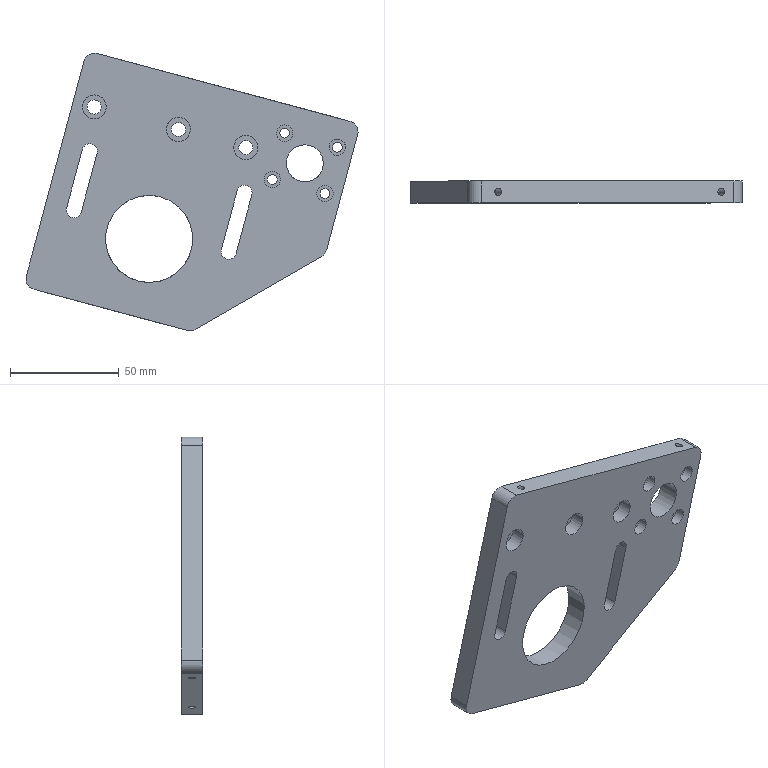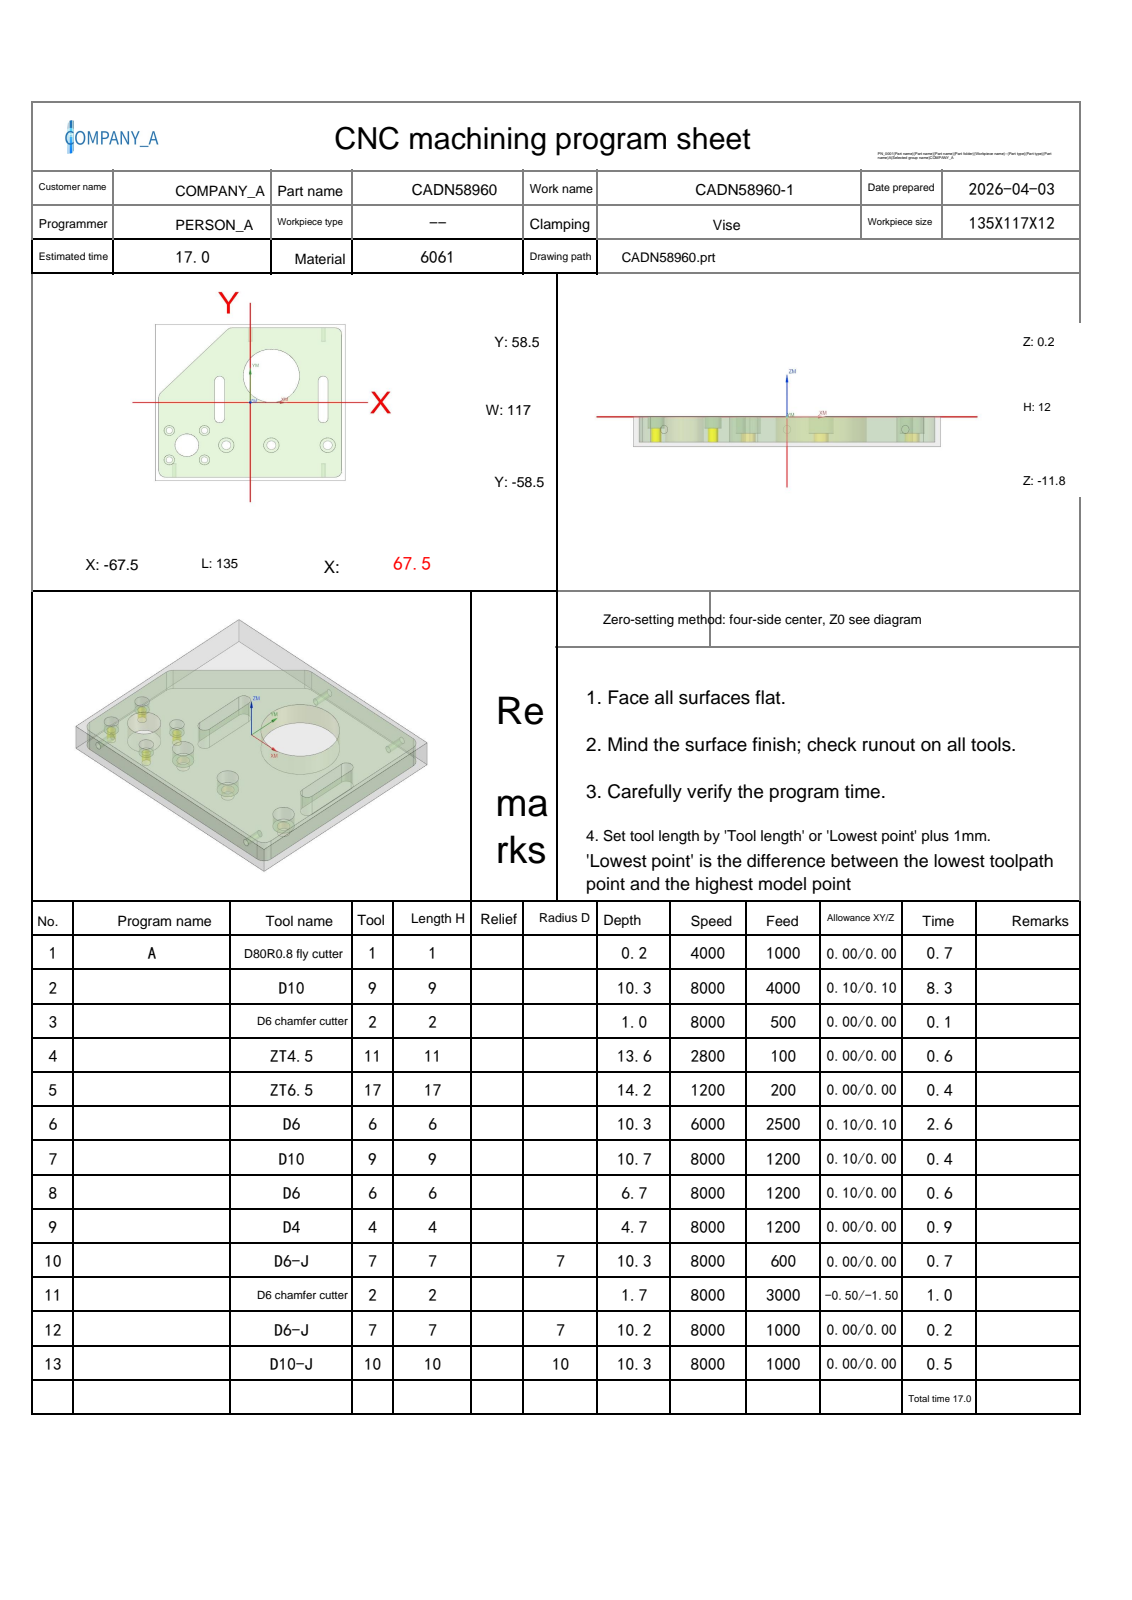NC program | NX | posted by the shop | part box 152.311 x 10 x 127.359 mm
Lines 40 to 980 of 4827:
N2 T09 M06
(D10  D=10. R=0. H=09 ce=0.10 di=0.10)
G00 G90 G54 X8.877 Y31.644 M03 S8000
G43 H09 Z10.2
M08
Z1.5
G02 X8.877 Y31.644 Z1.006 I3.69 J-2.576 F4000.
X8.877 Y31.644 Z.513 I3.69 J-2.576
X8.877 Y31.644 Z.019 I3.69 J-2.576
X8.877 Y31.644 Z-.474 I3.69 J-2.576
X9.115 Y31.955 Z-.481 I3.69 J-2.576
G01 X11.144 Y34.381
G02 X15. Y34.889 I3.856 J-14.392
X29.9 Y19.989 I0.0 J-14.9
X15. Y5.089 I-14.9 J0.0
X.1 Y19.989 I0.0 J14.9
X15. Y34.889 I14.9 J0.0
X16.098 Y34.848 I0.0 J-14.9
X17.014 Y33.997 I-.074 J-.997
G01 X17.925 Y27.835
G03 X18.474 Y27.084 I.989 J.147
G02 X22.9 Y19.989 I-3.474 J-7.095
X15. Y12.089 I-7.9 J0.0
X7.1 Y19.989 I0.0 J7.9
X12.241 Y27.391 I7.9 J0.0
X12.555 Y27.448 I.314 J-.843
X13.398 Y26.862 I0.0 J-.9
G01 X15.831 Y20.335
X15.84 Y20.311
G02 X15.9 Y19.989 I-.84 J-.322
X15. Y19.089 I-.9 J0.0
X14.1 Y19.989 I0.0 J.9
X15. Y20.889 I.9 J0.0
G01 X15.066 Y20.886
G02 X15.53 Y20.716 I-.066 J-.898
G03 X19.65 Y19.375 I4.12 J5.659
X25.309 Y22.255 I0.0 J7.
G01 Z.719
G00 Z3.
G01 X8.877 Y31.644 F6000.
G00 Z1.019
G02 X8.877 Y31.644 Z.526 I3.69 J-2.576 F4000.
X8.877 Y31.644 Z.032 I3.69 J-2.576
X8.877 Y31.644 Z-.462 I3.69 J-2.576
X8.877 Y31.644 Z-.955 I3.69 J-2.576
X9.115 Y31.955 Z-.962 I3.69 J-2.576
G01 X11.144 Y34.381
G02 X15. Y34.889 I3.856 J-14.392
X29.9 Y19.989 I0.0 J-14.9
X15. Y5.089 I-14.9 J0.0
X.1 Y19.989 I0.0 J14.9
X15. Y34.889 I14.9 J0.0
X16.098 Y34.848 I0.0 J-14.9
X17.014 Y33.997 I-.074 J-.997
G01 X17.925 Y27.835
G03 X18.474 Y27.084 I.989 J.147
G02 X22.9 Y19.989 I-3.474 J-7.095
X15. Y12.089 I-7.9 J0.0
X7.1 Y19.989 I0.0 J7.9
X12.241 Y27.391 I7.9 J0.0
X12.555 Y27.448 I.314 J-.843
X13.398 Y26.862 I0.0 J-.9
G01 X15.831 Y20.335
X15.84 Y20.311
G02 X15.9 Y19.989 I-.84 J-.322
X15. Y19.089 I-.9 J0.0
X14.1 Y19.989 I0.0 J.9
X15. Y20.889 I.9 J0.0
G01 X15.066 Y20.886
G02 X15.53 Y20.716 I-.066 J-.898
G03 X19.65 Y19.375 I4.12 J5.659
X25.309 Y22.255 I0.0 J7.
G01 Z.238
G00 Z2.519
G01 X8.877 Y31.644 F6000.
G00 Z.538
G02 X8.877 Y31.644 Z.045 I3.69 J-2.576 F4000.
X8.877 Y31.644 Z-.449 I3.69 J-2.576
X8.877 Y31.644 Z-.942 I3.69 J-2.576
X8.877 Y31.644 Z-1.436 I3.69 J-2.576
X9.115 Y31.955 Z-1.443 I3.69 J-2.576
G01 X11.144 Y34.381
G02 X15. Y34.889 I3.856 J-14.392
X29.9 Y19.989 I0.0 J-14.9
X15. Y5.089 I-14.9 J0.0
X.1 Y19.989 I0.0 J14.9
X15. Y34.889 I14.9 J0.0
X16.098 Y34.848 I0.0 J-14.9
X17.014 Y33.997 I-.074 J-.997
G01 X17.925 Y27.835
G03 X18.474 Y27.084 I.989 J.147
G02 X22.9 Y19.989 I-3.474 J-7.095
X15. Y12.089 I-7.9 J0.0
X7.1 Y19.989 I0.0 J7.9
X12.241 Y27.391 I7.9 J0.0
X12.555 Y27.448 I.314 J-.843
X13.398 Y26.862 I0.0 J-.9
G01 X15.831 Y20.335
X15.84 Y20.311
G02 X15.9 Y19.989 I-.84 J-.322
X15. Y19.089 I-.9 J0.0
X14.1 Y19.989 I0.0 J.9
X15. Y20.889 I.9 J0.0
G01 X15.066 Y20.886
G02 X15.53 Y20.716 I-.066 J-.898
G03 X19.65 Y19.375 I4.12 J5.659
X25.309 Y22.255 I0.0 J7.
G01 Z-.243
G00 Z2.038
G01 X8.877 Y31.644 F6000.
G00 Z.057
G02 X8.877 Y31.644 Z-.436 I3.69 J-2.576 F4000.
X8.877 Y31.644 Z-.93 I3.69 J-2.576
X8.877 Y31.644 Z-1.423 I3.69 J-2.576
X8.877 Y31.644 Z-1.917 I3.69 J-2.576
X9.115 Y31.955 Z-1.924 I3.69 J-2.576
G01 X11.144 Y34.381
G02 X15. Y34.889 I3.856 J-14.392
X29.9 Y19.989 I0.0 J-14.9
X15. Y5.089 I-14.9 J0.0
X.1 Y19.989 I0.0 J14.9
X15. Y34.889 I14.9 J0.0
X16.098 Y34.848 I0.0 J-14.9
X17.014 Y33.997 I-.074 J-.997
G01 X17.925 Y27.835
G03 X18.474 Y27.084 I.989 J.147
G02 X22.9 Y19.989 I-3.474 J-7.095
X15. Y12.089 I-7.9 J0.0
X7.1 Y19.989 I0.0 J7.9
X12.241 Y27.391 I7.9 J0.0
X12.555 Y27.448 I.314 J-.843
X13.398 Y26.862 I0.0 J-.9
G01 X15.831 Y20.335
X15.84 Y20.311
G02 X15.9 Y19.989 I-.84 J-.322
X15. Y19.089 I-.9 J0.0
X14.1 Y19.989 I0.0 J.9
X15. Y20.889 I.9 J0.0
G01 X15.066 Y20.886
G02 X15.53 Y20.716 I-.066 J-.898
G03 X19.65 Y19.375 I4.12 J5.659
X25.309 Y22.255 I0.0 J7.
G01 Z-.724
G00 Z1.557
G01 X8.877 Y31.644 F6000.
G00 Z-.424
G02 X8.877 Y31.644 Z-.917 I3.69 J-2.576 F4000.
X8.877 Y31.644 Z-1.411 I3.69 J-2.576
X8.877 Y31.644 Z-1.904 I3.69 J-2.576
X8.877 Y31.644 Z-2.398 I3.69 J-2.576
X9.115 Y31.955 Z-2.405 I3.69 J-2.576
G01 X11.144 Y34.381
G02 X15. Y34.889 I3.856 J-14.392
X29.9 Y19.989 I0.0 J-14.9
X15. Y5.089 I-14.9 J0.0
X.1 Y19.989 I0.0 J14.9
X15. Y34.889 I14.9 J0.0
X16.098 Y34.848 I0.0 J-14.9
X17.014 Y33.997 I-.074 J-.997
G01 X17.925 Y27.835
G03 X18.474 Y27.084 I.989 J.147
G02 X22.9 Y19.989 I-3.474 J-7.095
X15. Y12.089 I-7.9 J0.0
X7.1 Y19.989 I0.0 J7.9
X12.241 Y27.391 I7.9 J0.0
X12.555 Y27.448 I.314 J-.843
X13.398 Y26.862 I0.0 J-.9
G01 X15.831 Y20.335
X15.84 Y20.311
G02 X15.9 Y19.989 I-.84 J-.322
X15. Y19.089 I-.9 J0.0
X14.1 Y19.989 I0.0 J.9
X15. Y20.889 I.9 J0.0
G01 X15.066 Y20.886
G02 X15.53 Y20.716 I-.066 J-.898
G03 X19.65 Y19.375 I4.12 J5.659
X25.309 Y22.255 I0.0 J7.
G01 Z-1.205
G00 Z1.076
G01 X8.877 Y31.644 F6000.
G00 Z-.905
G02 X8.877 Y31.644 Z-1.398 I3.69 J-2.576 F4000.
X8.877 Y31.644 Z-1.892 I3.69 J-2.576
X8.877 Y31.644 Z-2.385 I3.69 J-2.576
X8.877 Y31.644 Z-2.879 I3.69 J-2.576
X9.115 Y31.955 Z-2.886 I3.69 J-2.576
G01 X11.144 Y34.381
G02 X15. Y34.889 I3.856 J-14.392
X29.9 Y19.989 I0.0 J-14.9
X15. Y5.089 I-14.9 J0.0
X.1 Y19.989 I0.0 J14.9
X15. Y34.889 I14.9 J0.0
X16.098 Y34.848 I0.0 J-14.9
X17.014 Y33.997 I-.074 J-.997
G01 X17.925 Y27.835
G03 X18.474 Y27.084 I.989 J.147
G02 X22.9 Y19.989 I-3.474 J-7.095
X15. Y12.089 I-7.9 J0.0
X7.1 Y19.989 I0.0 J7.9
X12.241 Y27.391 I7.9 J0.0
X12.555 Y27.448 I.314 J-.843
X13.398 Y26.862 I0.0 J-.9
G01 X15.831 Y20.335
X15.84 Y20.311
G02 X15.9 Y19.989 I-.84 J-.322
X15. Y19.089 I-.9 J0.0
X14.1 Y19.989 I0.0 J.9
X15. Y20.889 I.9 J0.0
G01 X15.066 Y20.886
G02 X15.53 Y20.716 I-.066 J-.898
G03 X19.65 Y19.375 I4.12 J5.659
X25.309 Y22.255 I0.0 J7.
G01 Z-1.686
G00 Z.595
G01 X8.877 Y31.644 F6000.
G00 Z-1.386
G02 X8.877 Y31.644 Z-1.879 I3.69 J-2.576 F4000.
X8.877 Y31.644 Z-2.373 I3.69 J-2.576
X8.877 Y31.644 Z-2.866 I3.69 J-2.576
X8.877 Y31.644 Z-3.36 I3.69 J-2.576
X9.115 Y31.955 Z-3.367 I3.69 J-2.576
G01 X11.144 Y34.381
G02 X15. Y34.889 I3.856 J-14.392
X29.9 Y19.989 I0.0 J-14.9
X15. Y5.089 I-14.9 J0.0
X.1 Y19.989 I0.0 J14.9
X15. Y34.889 I14.9 J0.0
X16.098 Y34.848 I0.0 J-14.9
X17.014 Y33.997 I-.074 J-.997
G01 X17.925 Y27.835
G03 X18.474 Y27.084 I.989 J.147
G02 X22.9 Y19.989 I-3.474 J-7.095
X15. Y12.089 I-7.9 J0.0
X7.1 Y19.989 I0.0 J7.9
X12.241 Y27.391 I7.9 J0.0
X12.555 Y27.448 I.314 J-.843
X13.398 Y26.862 I0.0 J-.9
G01 X15.831 Y20.335
X15.84 Y20.311
G02 X15.9 Y19.989 I-.84 J-.322
X15. Y19.089 I-.9 J0.0
X14.1 Y19.989 I0.0 J.9
X15. Y20.889 I.9 J0.0
G01 X15.066 Y20.886
G02 X15.53 Y20.716 I-.066 J-.898
G03 X19.65 Y19.375 I4.12 J5.659
X25.309 Y22.255 I0.0 J7.
G01 Z-2.167
G00 Z.114
G01 X8.877 Y31.644 F6000.
G00 Z-1.867
G02 X8.877 Y31.644 Z-2.36 I3.69 J-2.576 F4000.
X8.877 Y31.644 Z-2.854 I3.69 J-2.576
X8.877 Y31.644 Z-3.347 I3.69 J-2.576
X8.877 Y31.644 Z-3.841 I3.69 J-2.576
X9.115 Y31.955 Z-3.848 I3.69 J-2.576
G01 X11.144 Y34.381
G02 X15. Y34.889 I3.856 J-14.392
X29.9 Y19.989 I0.0 J-14.9
X15. Y5.089 I-14.9 J0.0
X.1 Y19.989 I0.0 J14.9
X15. Y34.889 I14.9 J0.0
X16.098 Y34.848 I0.0 J-14.9
X17.014 Y33.997 I-.074 J-.997
G01 X17.925 Y27.835
G03 X18.474 Y27.084 I.989 J.147
G02 X22.9 Y19.989 I-3.474 J-7.095
X15. Y12.089 I-7.9 J0.0
X7.1 Y19.989 I0.0 J7.9
X12.241 Y27.391 I7.9 J0.0
X12.555 Y27.448 I.314 J-.843
X13.398 Y26.862 I0.0 J-.9
G01 X15.831 Y20.335
X15.84 Y20.311
G02 X15.9 Y19.989 I-.84 J-.322
X15. Y19.089 I-.9 J0.0
X14.1 Y19.989 I0.0 J.9
X15. Y20.889 I.9 J0.0
G01 X15.066 Y20.886
G02 X15.53 Y20.716 I-.066 J-.898
G03 X19.65 Y19.375 I4.12 J5.659
X25.309 Y22.255 I0.0 J7.
G01 Z-2.648
G00 Z-.367
G01 X8.877 Y31.644 F6000.
G00 Z-2.348
G02 X8.877 Y31.644 Z-2.841 I3.69 J-2.576 F4000.
X8.877 Y31.644 Z-3.335 I3.69 J-2.576
X8.877 Y31.644 Z-3.828 I3.69 J-2.576
X8.877 Y31.644 Z-4.322 I3.69 J-2.576
X9.115 Y31.955 Z-4.329 I3.69 J-2.576
G01 X11.144 Y34.381
G02 X15. Y34.889 I3.856 J-14.392
X29.9 Y19.989 I0.0 J-14.9
X15. Y5.089 I-14.9 J0.0
X.1 Y19.989 I0.0 J14.9
X15. Y34.889 I14.9 J0.0
X16.098 Y34.848 I0.0 J-14.9
X17.014 Y33.997 I-.074 J-.997
G01 X17.925 Y27.835
G03 X18.474 Y27.084 I.989 J.147
G02 X22.9 Y19.989 I-3.474 J-7.095
X15. Y12.089 I-7.9 J0.0
X7.1 Y19.989 I0.0 J7.9
X12.241 Y27.391 I7.9 J0.0
X12.555 Y27.448 I.314 J-.843
X13.398 Y26.862 I0.0 J-.9
G01 X15.831 Y20.335
X15.84 Y20.311
G02 X15.9 Y19.989 I-.84 J-.322
X15. Y19.089 I-.9 J0.0
X14.1 Y19.989 I0.0 J.9
X15. Y20.889 I.9 J0.0
G01 X15.066 Y20.886
G02 X15.53 Y20.716 I-.066 J-.898
G03 X19.65 Y19.375 I4.12 J5.659
X25.309 Y22.255 I0.0 J7.
G01 Z-3.129
G00 Z-.848
G01 X8.877 Y31.644 F6000.
G00 Z-2.829
G02 X8.877 Y31.644 Z-3.322 I3.69 J-2.576 F4000.
X8.877 Y31.644 Z-3.816 I3.69 J-2.576
X8.877 Y31.644 Z-4.309 I3.69 J-2.576
X8.877 Y31.644 Z-4.803 I3.69 J-2.576
X9.115 Y31.955 Z-4.81 I3.69 J-2.576
G01 X11.144 Y34.381
G02 X15. Y34.889 I3.856 J-14.392
X29.9 Y19.989 I0.0 J-14.9
X15. Y5.089 I-14.9 J0.0
X.1 Y19.989 I0.0 J14.9
X15. Y34.889 I14.9 J0.0
X16.098 Y34.848 I0.0 J-14.9
X17.014 Y33.997 I-.074 J-.997
G01 X17.925 Y27.835
G03 X18.474 Y27.084 I.989 J.147
G02 X22.9 Y19.989 I-3.474 J-7.095
X15. Y12.089 I-7.9 J0.0
X7.1 Y19.989 I0.0 J7.9
X12.241 Y27.391 I7.9 J0.0
X12.555 Y27.448 I.314 J-.843
X13.398 Y26.862 I0.0 J-.9
G01 X15.831 Y20.335
X15.84 Y20.311
G02 X15.9 Y19.989 I-.84 J-.322
X15. Y19.089 I-.9 J0.0
X14.1 Y19.989 I0.0 J.9
X15. Y20.889 I.9 J0.0
G01 X15.066 Y20.886
G02 X15.53 Y20.716 I-.066 J-.898
G03 X19.65 Y19.375 I4.12 J5.659
X25.309 Y22.255 I0.0 J7.
G01 Z-3.61
G00 Z-1.329
G01 X8.877 Y31.644 F6000.
G00 Z-3.31
G02 X8.877 Y31.644 Z-3.803 I3.69 J-2.576 F4000.
X8.877 Y31.644 Z-4.297 I3.69 J-2.576
X8.877 Y31.644 Z-4.79 I3.69 J-2.576
X8.877 Y31.644 Z-5.284 I3.69 J-2.576
X9.115 Y31.955 Z-5.29 I3.69 J-2.576
G01 X11.144 Y34.381
G02 X15. Y34.889 I3.856 J-14.392
X29.9 Y19.989 I0.0 J-14.9
X15. Y5.089 I-14.9 J0.0
X.1 Y19.989 I0.0 J14.9
X15. Y34.889 I14.9 J0.0
X16.098 Y34.848 I0.0 J-14.9
X17.014 Y33.997 I-.074 J-.997
G01 X17.925 Y27.835
G03 X18.474 Y27.084 I.989 J.147
G02 X22.9 Y19.989 I-3.474 J-7.095
X15. Y12.089 I-7.9 J0.0
X7.1 Y19.989 I0.0 J7.9
X12.241 Y27.391 I7.9 J0.0
X12.555 Y27.448 I.314 J-.843
X13.398 Y26.862 I0.0 J-.9
G01 X15.831 Y20.335
X15.84 Y20.311
G02 X15.9 Y19.989 I-.84 J-.322
X15. Y19.089 I-.9 J0.0
X14.1 Y19.989 I0.0 J.9
X15. Y20.889 I.9 J0.0
G01 X15.066 Y20.886
G02 X15.53 Y20.716 I-.066 J-.898
G03 X19.65 Y19.375 I4.12 J5.659
X25.309 Y22.255 I0.0 J7.
G01 Z-4.09
G00 Z-1.81
G01 X8.877 Y31.644 F6000.
G00 Z-3.79
G02 X8.877 Y31.644 Z-4.284 I3.69 J-2.576 F4000.
X8.877 Y31.644 Z-4.778 I3.69 J-2.576
X8.877 Y31.644 Z-5.271 I3.69 J-2.576
X8.877 Y31.644 Z-5.765 I3.69 J-2.576
X9.115 Y31.955 Z-5.771 I3.69 J-2.576
G01 X11.144 Y34.381
G02 X15. Y34.889 I3.856 J-14.392
X29.9 Y19.989 I0.0 J-14.9
X15. Y5.089 I-14.9 J0.0
X.1 Y19.989 I0.0 J14.9
X15. Y34.889 I14.9 J0.0
X16.098 Y34.848 I0.0 J-14.9
X17.014 Y33.997 I-.074 J-.997
G01 X17.925 Y27.835
G03 X18.474 Y27.084 I.989 J.147
G02 X22.9 Y19.989 I-3.474 J-7.095
X15. Y12.089 I-7.9 J0.0
X7.1 Y19.989 I0.0 J7.9
X12.241 Y27.391 I7.9 J0.0
X12.555 Y27.448 I.314 J-.843
X13.398 Y26.862 I0.0 J-.9
G01 X15.831 Y20.335
X15.84 Y20.311
G02 X15.9 Y19.989 I-.84 J-.322
X15. Y19.089 I-.9 J0.0
X14.1 Y19.989 I0.0 J.9
X15. Y20.889 I.9 J0.0
G01 X15.066 Y20.886
G02 X15.53 Y20.716 I-.066 J-.898
G03 X19.65 Y19.375 I4.12 J5.659
X25.309 Y22.255 I0.0 J7.
G01 Z-4.571
G00 Z-2.29
G01 X8.877 Y31.644 F6000.
G00 Z-4.271
G02 X8.877 Y31.644 Z-4.765 I3.69 J-2.576 F4000.
X8.877 Y31.644 Z-5.258 I3.69 J-2.576
X8.877 Y31.644 Z-5.752 I3.69 J-2.576
X8.877 Y31.644 Z-6.246 I3.69 J-2.576
X9.115 Y31.955 Z-6.252 I3.69 J-2.576
G01 X11.144 Y34.381
G02 X15. Y34.889 I3.856 J-14.392
X29.9 Y19.989 I0.0 J-14.9
X15. Y5.089 I-14.9 J0.0
X.1 Y19.989 I0.0 J14.9
X15. Y34.889 I14.9 J0.0
X16.098 Y34.848 I0.0 J-14.9
X17.014 Y33.997 I-.074 J-.997
G01 X17.925 Y27.835
G03 X18.474 Y27.084 I.989 J.147
G02 X22.9 Y19.989 I-3.474 J-7.095
X15. Y12.089 I-7.9 J0.0
X7.1 Y19.989 I0.0 J7.9
X12.241 Y27.391 I7.9 J0.0
X12.555 Y27.448 I.314 J-.843
X13.398 Y26.862 I0.0 J-.9
G01 X15.831 Y20.335
X15.84 Y20.311
G02 X15.9 Y19.989 I-.84 J-.322
X15. Y19.089 I-.9 J0.0
X14.1 Y19.989 I0.0 J.9
X15. Y20.889 I.9 J0.0
G01 X15.066 Y20.886
G02 X15.53 Y20.716 I-.066 J-.898
G03 X19.65 Y19.375 I4.12 J5.659
X25.309 Y22.255 I0.0 J7.
G01 Z-5.052
G00 Z-2.771
G01 X8.877 Y31.644 F6000.
G00 Z-4.752
G02 X8.877 Y31.644 Z-5.246 I3.69 J-2.576 F4000.
X8.877 Y31.644 Z-5.739 I3.69 J-2.576
X8.877 Y31.644 Z-6.233 I3.69 J-2.576
X8.877 Y31.644 Z-6.727 I3.69 J-2.576
X9.115 Y31.955 Z-6.733 I3.69 J-2.576
G01 X11.144 Y34.381
G02 X15. Y34.889 I3.856 J-14.392
X29.9 Y19.989 I0.0 J-14.9
X15. Y5.089 I-14.9 J0.0
X.1 Y19.989 I0.0 J14.9
X15. Y34.889 I14.9 J0.0
X16.098 Y34.848 I0.0 J-14.9
X17.014 Y33.997 I-.074 J-.997
G01 X17.925 Y27.835
G03 X18.474 Y27.084 I.989 J.147
G02 X22.9 Y19.989 I-3.474 J-7.095
X15. Y12.089 I-7.9 J0.0
X7.1 Y19.989 I0.0 J7.9
X12.241 Y27.391 I7.9 J0.0
X12.555 Y27.448 I.314 J-.843
X13.398 Y26.862 I0.0 J-.9
G01 X15.831 Y20.335
X15.84 Y20.311
G02 X15.9 Y19.989 I-.84 J-.322
X15. Y19.089 I-.9 J0.0
X14.1 Y19.989 I0.0 J.9
X15. Y20.889 I.9 J0.0
G01 X15.066 Y20.886
G02 X15.53 Y20.716 I-.066 J-.898
G03 X19.65 Y19.375 I4.12 J5.659
X25.309 Y22.255 I0.0 J7.
G01 Z-5.533
G00 Z-3.252
G01 X8.877 Y31.644 F6000.
G00 Z-5.233
G02 X8.877 Y31.644 Z-5.727 I3.69 J-2.576 F4000.
X8.877 Y31.644 Z-6.22 I3.69 J-2.576
X8.877 Y31.644 Z-6.714 I3.69 J-2.576
X8.877 Y31.644 Z-7.207 I3.69 J-2.576
X9.115 Y31.955 Z-7.214 I3.69 J-2.576
G01 X11.144 Y34.381
G02 X15. Y34.889 I3.856 J-14.392
X29.9 Y19.989 I0.0 J-14.9
X15. Y5.089 I-14.9 J0.0
X.1 Y19.989 I0.0 J14.9
X15. Y34.889 I14.9 J0.0
X16.098 Y34.848 I0.0 J-14.9
X17.014 Y33.997 I-.074 J-.997
G01 X17.925 Y27.835
G03 X18.474 Y27.084 I.989 J.147
G02 X22.9 Y19.989 I-3.474 J-7.095
X15. Y12.089 I-7.9 J0.0
X7.1 Y19.989 I0.0 J7.9
X12.241 Y27.391 I7.9 J0.0
X12.555 Y27.448 I.314 J-.843
X13.398 Y26.862 I0.0 J-.9
G01 X15.831 Y20.335
X15.84 Y20.311
G02 X15.9 Y19.989 I-.84 J-.322
X15. Y19.089 I-.9 J0.0
X14.1 Y19.989 I0.0 J.9
X15. Y20.889 I.9 J0.0
G01 X15.066 Y20.886
G02 X15.53 Y20.716 I-.066 J-.898
G03 X19.65 Y19.375 I4.12 J5.659
X25.309 Y22.255 I0.0 J7.
G01 Z-6.014
G00 Z-3.733
G01 X8.877 Y31.644 F6000.
G00 Z-5.714
G02 X8.877 Y31.644 Z-6.208 I3.69 J-2.576 F4000.
X8.877 Y31.644 Z-6.701 I3.69 J-2.576
X8.877 Y31.644 Z-7.195 I3.69 J-2.576
X8.877 Y31.644 Z-7.688 I3.69 J-2.576
X9.115 Y31.955 Z-7.695 I3.69 J-2.576
G01 X11.144 Y34.381
G02 X15. Y34.889 I3.856 J-14.392
X29.9 Y19.989 I0.0 J-14.9
X15. Y5.089 I-14.9 J0.0
X.1 Y19.989 I0.0 J14.9
X15. Y34.889 I14.9 J0.0
X16.098 Y34.848 I0.0 J-14.9
X17.014 Y33.997 I-.074 J-.997
G01 X17.925 Y27.835
G03 X18.474 Y27.084 I.989 J.147
G02 X22.9 Y19.989 I-3.474 J-7.095
X15. Y12.089 I-7.9 J0.0
X7.1 Y19.989 I0.0 J7.9
X12.241 Y27.391 I7.9 J0.0
X12.555 Y27.448 I.314 J-.843
X13.398 Y26.862 I0.0 J-.9
G01 X15.831 Y20.335
X15.84 Y20.311
G02 X15.9 Y19.989 I-.84 J-.322
X15. Y19.089 I-.9 J0.0
X14.1 Y19.989 I0.0 J.9
X15. Y20.889 I.9 J0.0
G01 X15.066 Y20.886
G02 X15.53 Y20.716 I-.066 J-.898
G03 X19.65 Y19.375 I4.12 J5.659
X25.309 Y22.255 I0.0 J7.
G01 Z-6.495
G00 Z-4.214
G01 X8.877 Y31.644 F6000.
G00 Z-6.195
G02 X8.877 Y31.644 Z-6.689 I3.69 J-2.576 F4000.
X8.877 Y31.644 Z-7.182 I3.69 J-2.576
X8.877 Y31.644 Z-7.676 I3.69 J-2.576
X8.877 Y31.644 Z-8.169 I3.69 J-2.576
X9.115 Y31.955 Z-8.176 I3.69 J-2.576
G01 X11.144 Y34.381
G02 X15. Y34.889 I3.856 J-14.392
X29.9 Y19.989 I0.0 J-14.9
X15. Y5.089 I-14.9 J0.0
X.1 Y19.989 I0.0 J14.9
X15. Y34.889 I14.9 J0.0
X16.098 Y34.848 I0.0 J-14.9
X17.014 Y33.997 I-.074 J-.997
G01 X17.925 Y27.835
G03 X18.474 Y27.084 I.989 J.147
G02 X22.9 Y19.989 I-3.474 J-7.095
X15. Y12.089 I-7.9 J0.0
X7.1 Y19.989 I0.0 J7.9
X12.241 Y27.391 I7.9 J0.0
X12.555 Y27.448 I.314 J-.843
X13.398 Y26.862 I0.0 J-.9
G01 X15.831 Y20.335
X15.84 Y20.311
G02 X15.9 Y19.989 I-.84 J-.322
X15. Y19.089 I-.9 J0.0
X14.1 Y19.989 I0.0 J.9
X15. Y20.889 I.9 J0.0
G01 X15.066 Y20.886
G02 X15.53 Y20.716 I-.066 J-.898
G03 X19.65 Y19.375 I4.12 J5.659
X25.309 Y22.255 I0.0 J7.
G01 Z-6.976
G00 Z-4.695
G01 X8.877 Y31.644 F6000.
G00 Z-6.676
G02 X8.877 Y31.644 Z-7.17 I3.69 J-2.576 F4000.
X8.877 Y31.644 Z-7.663 I3.69 J-2.576
X8.877 Y31.644 Z-8.157 I3.69 J-2.576
X8.877 Y31.644 Z-8.65 I3.69 J-2.576
X9.115 Y31.955 Z-8.657 I3.69 J-2.576
G01 X11.144 Y34.381
G02 X15. Y34.889 I3.856 J-14.392
X29.9 Y19.989 I0.0 J-14.9
X15. Y5.089 I-14.9 J0.0
X.1 Y19.989 I0.0 J14.9
X15. Y34.889 I14.9 J0.0
X16.098 Y34.848 I0.0 J-14.9
X17.014 Y33.997 I-.074 J-.997
G01 X17.925 Y27.835
G03 X18.474 Y27.084 I.989 J.147
G02 X22.9 Y19.989 I-3.474 J-7.095
X15. Y12.089 I-7.9 J0.0
X7.1 Y19.989 I0.0 J7.9
X12.241 Y27.391 I7.9 J0.0
X12.555 Y27.448 I.314 J-.843
X13.398 Y26.862 I0.0 J-.9
G01 X15.831 Y20.335
X15.84 Y20.311
G02 X15.9 Y19.989 I-.84 J-.322
X15. Y19.089 I-.9 J0.0
X14.1 Y19.989 I0.0 J.9
X15. Y20.889 I.9 J0.0
G01 X15.066 Y20.886
G02 X15.53 Y20.716 I-.066 J-.898
G03 X19.65 Y19.375 I4.12 J5.659
X25.309 Y22.255 I0.0 J7.
G01 Z-7.457
G00 Z-5.176
G01 X8.877 Y31.644 F6000.
G00 Z-7.157
G02 X8.877 Y31.644 Z-7.651 I3.69 J-2.576 F4000.
X8.877 Y31.644 Z-8.144 I3.69 J-2.576
X8.877 Y31.644 Z-8.638 I3.69 J-2.576
X8.877 Y31.644 Z-9.131 I3.69 J-2.576
X9.115 Y31.955 Z-9.138 I3.69 J-2.576
G01 X11.144 Y34.381
G02 X15. Y34.889 I3.856 J-14.392
X29.9 Y19.989 I0.0 J-14.9
X15. Y5.089 I-14.9 J0.0
X.1 Y19.989 I0.0 J14.9
X15. Y34.889 I14.9 J0.0
X16.098 Y34.848 I0.0 J-14.9
X17.014 Y33.997 I-.074 J-.997
G01 X17.925 Y27.835
G03 X18.474 Y27.084 I.989 J.147
G02 X22.9 Y19.989 I-3.474 J-7.095
X15. Y12.089 I-7.9 J0.0
X7.1 Y19.989 I0.0 J7.9
X12.241 Y27.391 I7.9 J0.0
X12.555 Y27.448 I.314 J-.843
X13.398 Y26.862 I0.0 J-.9
G01 X15.831 Y20.335
X15.84 Y20.311
G02 X15.9 Y19.989 I-.84 J-.322
X15. Y19.089 I-.9 J0.0
X14.1 Y19.989 I0.0 J.9
X15. Y20.889 I.9 J0.0
G01 X15.066 Y20.886
G02 X15.53 Y20.716 I-.066 J-.898
G03 X19.65 Y19.375 I4.12 J5.659
X25.309 Y22.255 I0.0 J7.
G01 Z-7.938
G00 Z-5.657
G01 X8.877 Y31.644 F6000.
G00 Z-7.638
G02 X8.877 Y31.644 Z-8.132 I3.69 J-2.576 F4000.
X8.877 Y31.644 Z-8.625 I3.69 J-2.576
X8.877 Y31.644 Z-9.119 I3.69 J-2.576
X8.877 Y31.644 Z-9.612 I3.69 J-2.576
X9.115 Y31.955 Z-9.619 I3.69 J-2.576
G01 X11.144 Y34.381
G02 X15. Y34.889 I3.856 J-14.392
X29.9 Y19.989 I0.0 J-14.9
X15. Y5.089 I-14.9 J0.0
X.1 Y19.989 I0.0 J14.9
X15. Y34.889 I14.9 J0.0
X16.098 Y34.848 I0.0 J-14.9
X17.014 Y33.997 I-.074 J-.997
G01 X17.925 Y27.835
G03 X18.474 Y27.084 I.989 J.147
G02 X22.9 Y19.989 I-3.474 J-7.095
X15. Y12.089 I-7.9 J0.0
X7.1 Y19.989 I0.0 J7.9
X12.241 Y27.391 I7.9 J0.0
X12.555 Y27.448 I.314 J-.843
X13.398 Y26.862 I0.0 J-.9
G01 X15.831 Y20.335
X15.84 Y20.311
G02 X15.9 Y19.989 I-.84 J-.322
X15. Y19.089 I-.9 J0.0
X14.1 Y19.989 I0.0 J.9
X15. Y20.889 I.9 J0.0
G01 X15.066 Y20.886
G02 X15.53 Y20.716 I-.066 J-.898
G03 X19.65 Y19.375 I4.12 J5.659
X25.309 Y22.255 I0.0 J7.
G01 Z-8.419
G00 Z-6.138
G01 X8.877 Y31.644 F6000.
G00 Z-8.119
G02 X8.877 Y31.644 Z-8.613 I3.69 J-2.576 F4000.
X8.877 Y31.644 Z-9.106 I3.69 J-2.576
X8.877 Y31.644 Z-9.6 I3.69 J-2.576
X8.877 Y31.644 Z-10.093 I3.69 J-2.576
X9.115 Y31.955 Z-10.1 I3.69 J-2.576
G01 X11.144 Y34.381
G02 X15. Y34.889 I3.856 J-14.392
X29.9 Y19.989 I0.0 J-14.9
X15. Y5.089 I-14.9 J0.0
X.1 Y19.989 I0.0 J14.9
X15. Y34.889 I14.9 J0.0
X16.098 Y34.848 I0.0 J-14.9
X17.014 Y33.997 I-.074 J-.997
G01 X17.925 Y27.835
G03 X18.474 Y27.084 I.989 J.147
G02 X22.9 Y19.989 I-3.474 J-7.095
X15. Y12.089 I-7.9 J0.0
X7.1 Y19.989 I0.0 J7.9
X12.171 Y27.365 I7.9 J0.0
X12.493 Y27.424 I.322 J-.84
X13.357 Y26.775 I0.0 J-.9
G01 X14.72 Y22.081
G03 X15.607 Y20.653 I2.987 J.867
G02 X15.9 Y19.989 I-.607 J-.664
X15. Y19.089 I-.9 J0.0
X14.1 Y19.989 I0.0 J.9
X15. Y20.889 I.9 J0.0
G01 X15.066 Y20.886
G02 X15.53 Y20.716 I-.066 J-.898
G03 X19.65 Y19.375 I4.12 J5.659
X25.309 Y22.255 I0.0 J7.
G01 Z-8.9
G00 Z10.2
X-57.175 Y70.5
Z.719
G01 Z-.481
Y66.
G03 X-50.175 Y59. I7. J0.0
G01 X-21.036
X-20.904 Y59.132
G02 X-12.772 Y62.5 I8.132 J-8.132
G01 X60.
G02 X71.5 Y51. I0.0 J-11.5
G01 Y23.495
Y4.133
Y-48.811
Y-51.
G02 X60.84 Y-62.469 I-11.5 J0.0
X59.999 Y-62.5 I-.841 J11.47
G01 X59.952
X-60.
G02 X-71.5 Y-51. I0.0 J11.5
G01 Y-39.916
Y3.772
G02 X-68.132 Y11.904 I11.5 J0.0
G01 X-68. Y12.036
Y58.5
G02 X-67.5 Y59. I.5 J0.0
G01 X-45.175
G02 X-44.203 Y58.238 I0.0 J-1.
G01 X-42.861 Y52.762
G03 X-41.89 Y52. I.971 J.238
G01 X-30.447
G02 X-29.45 Y51. I-.003 J-1.
X-29.74 Y50.295 I-1. J0.0
G01 X-34.715 Y45.32
G02 X-35.422 Y45.027 I-.707 J.707
G01 X-35.528 Y45.033
X-37.498 Y45.243
X-37.604 Y45.248
G03 X-37.986 Y45.172 I0.0 J-1.
G01 X-43.067 Y43.068
G02 X-44.023 Y42.878 I-.957 J2.31
X-46.523 Y45.378 I0.0 J2.5
X-44.98 Y47.687 I2.5 J0.0
G01 X-38.846 Y50.228
G02 X-37.889 Y50.418 I.957 J-2.31
X-35.389 Y47.918 I0.0 J-2.5
X-35.975 Y46.31 I-2.5 J0.0
G03 X-36.209 Y45.716 I.766 J-.643
G01 X-36.287 Y44.115
G02 X-36.579 Y43.457 I-.999 J.049
G01 X-58.947 Y21.089
G03 X-59.175 Y20.538 I.551 J-.551
X-59.13 Y20.277 I.779 J0.0
G01 X-58.998 Y19.906
G03 X-58.602 Y19.627 I.396 J.141
X-58.305 Y19.75 I0.0 J.42
G01 X-47.115 Y30.941
X-45.355 Y32.701
X-19.914 Y58.142
G02 X-12.772 Y61.1 I7.142 J-7.142
G01 X60.
G02 X70.1 Y51. I0.0 J-10.1
G01 Y23.495
Y4.133
Y-48.811
Y-51.
G02 X60.738 Y-61.073 I-10.1 J0.0
X59.999 Y-61.1 I-.739 J10.074
G01 X59.955
X-60.
G02 X-70.1 Y-51. I0.0 J10.1
G01 Y-39.916
Y3.772
G02 X-67.142 Y10.914 I10.1 J0.0
G01 X-58.305 Y19.75
G03 X-58.182 Y20.047 I-.297 J.297
X-58.461 Y20.443 I-.42 J0.0
G01 X-59.084 Y20.665
X-59.218 Y20.688
G03 X-59.441 Y20.62 I0.0 J-.4
G02 X-60. Y20.45 I-.559 J.829
X-61. Y21.447 I0.0 J1.
G01 Y28.482
G02 X-60.628 Y29.26 I1. J0.0
G01 X-59.087 Y30.505
G03 X-58.792 Y30.9 I-.628 J.778
G01 X-56.687 Y35.98
G02 X-54.378 Y37.523 I2.31 J-.957
X-51.878 Y35.023 I0.0 J-2.5
X-52.068 Y34.067 I-2.5 J0.0
G01 X-54.609 Y27.933
G02 X-56.918 Y26.389 I-2.31 J.957
X-59.409 Y28.673 I0.0 J2.5
G03 X-59.664 Y29.258 I-.996 J-.086
G01 X-60.741 Y30.446
G02 X-61. Y31.118 I.741 J.672
G01 Y51.003
G02 X-60.003 Y52. I1. J-.003
G01 X-48.594
G02 X-47.598 Y51.084 I0.0 J-1.
G01 X-47.132 Y45.506
G03 X-46.743 Y44.795 I.997 J.084
G02 X-46.349 Y44. I-.607 J-.795
X-46.64 Y43.295 I-1. J0.0
G01 X-52.295 Y37.64
G02 X-53. Y37.349 I-.705 J.71
X-54. Y38.346 I0.0 J1.
G01 Y44.003
G02 X-53.003 Y45. I1. J-.003
G01 X-47.346
G02 X-47.087 Y44.965 I-.003 J-1.
X-46.656 Y44.721 I-.262 J-.965
G03 X-41.807 Y42.769 I4.85 J5.048
X-36.759 Y44.919 I0.0 J7.
G01 Y70.5
Z.719
G00 Z3.
G01 X-57.175 F6000.
G00 Z.238
G01 Z-.962 F4000.
Y66.
G03 X-50.175 Y59. I7. J0.0
G01 X-21.036
X-20.904 Y59.132
G02 X-12.772 Y62.5 I8.132 J-8.132
G01 X60.
G02 X71.5 Y51. I0.0 J-11.5
G01 Y-51.
G02 X60.839 Y-62.469 I-11.5 J0.0
X59.999 Y-62.5 I-.841 J11.471
G01 X59.952
X-60.
G02 X-71.5 Y-51. I0.0 J11.5
G01 Y3.772
G02 X-68.132 Y11.904 I11.5 J0.0
G01 X-68. Y12.036
Y58.5
G02 X-67.5 Y59. I.5 J0.0
G01 X-45.175
G02 X-44.203 Y58.238 I0.0 J-1.
G01 X-42.861 Y52.762
G03 X-41.89 Y52. I.971 J.238
G01 X-30.446
G02 X-29.45 Y51. I-.003 J-1.
X-29.74 Y50.295 I-1. J0.0
G01 X-34.715 Y45.32
G02 X-35.422 Y45.027 I-.707 J.707
G01 X-35.528 Y45.033
X-37.498 Y45.243
X-37.604 Y45.248
G03 X-37.986 Y45.172 I0.0 J-1.
G01 X-43.067 Y43.068
G02 X-44.023 Y42.878 I-.957 J2.31
X-46.523 Y45.378 I0.0 J2.5
X-44.98 Y47.687 I2.5 J0.0
G01 X-38.846 Y50.228
G02 X-37.889 Y50.418 I.957 J-2.31
X-35.389 Y47.918 I0.0 J-2.5
X-35.975 Y46.31 I-2.5 J0.0
G03 X-36.209 Y45.716 I.766 J-.643
G01 X-36.287 Y44.115
G02 X-36.579 Y43.457 I-.999 J.049
G01 X-52.457 Y27.579
G02 X-53.115 Y27.287 I-.707 J.707
G01 X-54.716 Y27.209
G03 X-55.31 Y26.976 I.049 J-.999
G02 X-56.918 Y26.389 I-1.609 J1.914
X-59.418 Y28.889 I0.0 J2.5
X-59.228 Y29.846 I2.5 J0.0
G01 X-56.687 Y35.98
G02 X-54.378 Y37.523 I2.31 J-.957
X-51.878 Y35.023 I0.0 J-2.5
X-52.068 Y34.067 I-2.5 J0.0
G01 X-54.172 Y28.986
G03 X-54.248 Y28.604 I.924 J-.383
G01 X-54.243 Y28.498
X-54.033 Y26.528
X-54.027 Y26.422
G02 X-54.32 Y25.715 I-1. J0.0
G01 X-58.947 Y21.088
G03 X-59.175 Y20.538 I.551 J-.551
X-59.13 Y20.276 I.779 J0.0
G01 X-58.998 Y19.906
G03 X-58.602 Y19.627 I.396 J.141
X-58.305 Y19.75 I0.0 J.42
G01 X-19.914 Y58.142
G02 X-12.772 Y61.1 I7.142 J-7.142
G01 X60.
G02 X70.1 Y51. I0.0 J-10.1
G01 Y-51.
G02 X60.737 Y-61.073 I-10.1 J0.0
X59.999 Y-61.1 I-.738 J10.074
G01 X59.955
X-60.
G02 X-70.1 Y-51. I0.0 J10.1
G01 Y3.772
G02 X-67.142 Y10.914 I10.1 J0.0
G01 X-58.305 Y19.75
G03 X-58.182 Y20.047 I-.297 J.297
X-58.461 Y20.443 I-.42 J0.0
G01 X-59.084 Y20.665
X-59.218 Y20.688
G03 X-59.442 Y20.62 I0.0 J-.4